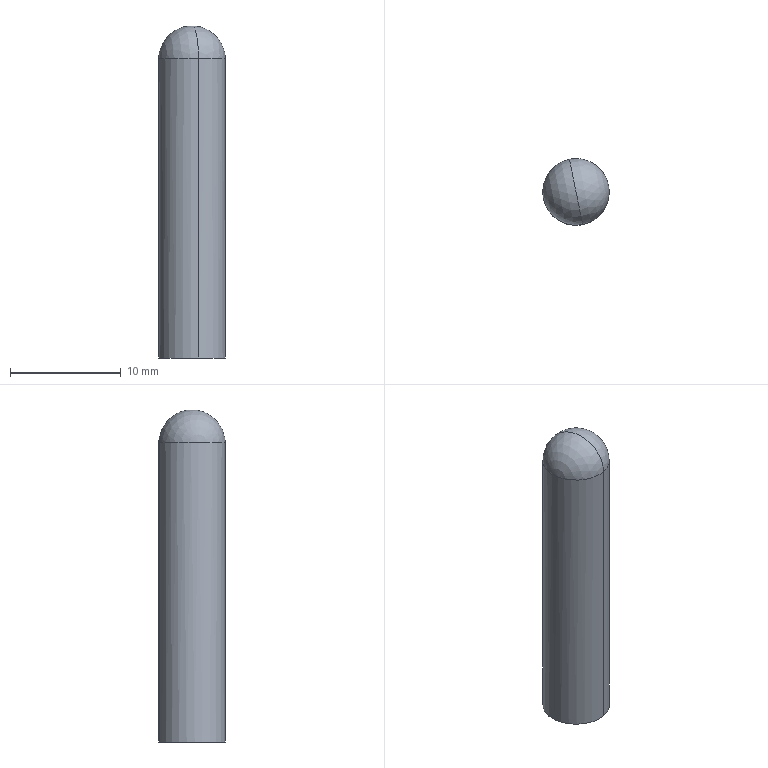Part | SolidWorks | features BaseBody 1 | 1 solid | 9 faces | box 6 x 6 x 30 mm | volume 732.824 mm3 | cylinder 4 | sphere 2 | cone 2 | plane 1 | commonest cylinder face diameters 2.5 x2 6 x2
STEP:
#1=CARTESIAN_POINT('',(-732.541,722.355,502.732));
#2=VERTEX_POINT('',#1);
#3=CARTESIAN_POINT('',(-732.541,722.355,529.732));
#4=VERTEX_POINT('',#3);
#5=CARTESIAN_POINT('',(-732.541,722.355,502.732));
#6=DIRECTION('',(0.,0.,1.));
#7=VECTOR('',#6,1000.);
#8=LINE('',#5,#7);
#9=EDGE_CURVE('',#2,#4,#8,.T.);
#10=ORIENTED_EDGE('',*,*,#9,.F.);
#11=CARTESIAN_POINT('',(-733.72,728.238,502.732));
#12=VERTEX_POINT('',#11);
#13=CARTESIAN_POINT('',(-733.131,725.297,502.732));
#14=DIRECTION('',(0.,0.,1.));
#15=DIRECTION('',(0.1964,-0.9805,0.));
#16=AXIS2_PLACEMENT_3D('',#13,#14,#15);
#17=CIRCLE('',#16,3.);
#18=EDGE_CURVE('',#2,#12,#17,.T.);
#19=ORIENTED_EDGE('',*,*,#18,.T.);
#20=CARTESIAN_POINT('',(-733.72,728.238,529.732));
#21=VERTEX_POINT('',#20);
#22=CARTESIAN_POINT('',(-733.72,728.238,529.732));
#23=DIRECTION('',(0.,0.,-1.));
#24=VECTOR('',#23,1000.);
#25=LINE('',#22,#24);
#26=EDGE_CURVE('',#21,#12,#25,.T.);
#27=ORIENTED_EDGE('',*,*,#26,.F.);
#28=CARTESIAN_POINT('',(-733.131,725.297,529.732));
#29=DIRECTION('',(0.,0.,-1.));
#30=DIRECTION('',(-0.1964,0.9805,0.));
#31=AXIS2_PLACEMENT_3D('',#28,#29,#30);
#32=CIRCLE('',#31,3.);
#33=EDGE_CURVE('',#21,#4,#32,.T.);
#34=ORIENTED_EDGE('',*,*,#33,.T.);
#35=EDGE_LOOP('',(#10,#19,#27,#34));
#36=FACE_OUTER_BOUND('',#35,.T.);
#37=CARTESIAN_POINT('',(-733.131,725.297,532.732));
#38=DIRECTION('',(0.,0.,-1.));
#39=DIRECTION('',(0.1964,-0.9805,0.));
#40=AXIS2_PLACEMENT_3D('',#37,#38,#39);
#41=CYLINDRICAL_SURFACE('',#40,3.);
#42=ADVANCED_FACE('',(#36),#41,.T.);
#43=CARTESIAN_POINT('',(-733.131,725.297,529.732));
#44=DIRECTION('',(0.9805,0.1964,0.));
#45=DIRECTION('',(-0.1964,0.9805,0.));
#46=AXIS2_PLACEMENT_3D('',#43,#44,#45);
#47=CIRCLE('',#46,3.);
#48=EDGE_CURVE('',#21,#4,#47,.T.);
#49=ORIENTED_EDGE('',*,*,#48,.T.);
#50=ORIENTED_EDGE('',*,*,#33,.F.);
#51=EDGE_LOOP('',(#49,#50));
#52=FACE_OUTER_BOUND('',#51,.T.);
#53=CARTESIAN_POINT('',(-733.131,725.297,529.732));
#54=DIRECTION('',(-0.9805,-0.1964,0.));
#55=DIRECTION('',(-0.1964,0.9805,0.));
#56=AXIS2_PLACEMENT_3D('',#53,#54,#55);
#57=SPHERICAL_SURFACE('',#56,3.);
#58=ADVANCED_FACE('',(#52),#57,.T.);
#59=CARTESIAN_POINT('',(-733.131,725.297,529.732));
#60=DIRECTION('',(0.,0.,-1.));
#61=DIRECTION('',(0.1964,-0.9805,0.));
#62=AXIS2_PLACEMENT_3D('',#59,#60,#61);
#63=CIRCLE('',#62,3.);
#64=EDGE_CURVE('',#4,#21,#63,.T.);
#65=ORIENTED_EDGE('',*,*,#64,.F.);
#66=ORIENTED_EDGE('',*,*,#48,.F.);
#67=EDGE_LOOP('',(#65,#66));
#68=FACE_OUTER_BOUND('',#67,.T.);
#69=CARTESIAN_POINT('',(-733.131,725.297,529.732));
#70=DIRECTION('',(-0.9805,-0.1964,0.));
#71=DIRECTION('',(-0.1964,0.9805,0.));
#72=AXIS2_PLACEMENT_3D('',#69,#70,#71);
#73=SPHERICAL_SURFACE('',#72,3.);
#74=ADVANCED_FACE('',(#68),#73,.T.);
#75=ORIENTED_EDGE('',*,*,#26,.T.);
#76=CARTESIAN_POINT('',(-733.131,725.297,502.732));
#77=DIRECTION('',(0.,0.,1.));
#78=DIRECTION('',(-0.1964,0.9805,0.));
#79=AXIS2_PLACEMENT_3D('',#76,#77,#78);
#80=CIRCLE('',#79,3.);
#81=EDGE_CURVE('',#12,#2,#80,.T.);
#82=ORIENTED_EDGE('',*,*,#81,.T.);
#83=ORIENTED_EDGE('',*,*,#9,.T.);
#84=ORIENTED_EDGE('',*,*,#64,.T.);
#85=EDGE_LOOP('',(#75,#82,#83,#84));
#86=FACE_OUTER_BOUND('',#85,.T.);
#87=CARTESIAN_POINT('',(-733.131,725.297,532.732));
#88=DIRECTION('',(0.,0.,-1.));
#89=DIRECTION('',(0.1964,-0.9805,0.));
#90=AXIS2_PLACEMENT_3D('',#87,#88,#89);
#91=CYLINDRICAL_SURFACE('',#90,3.);
#92=ADVANCED_FACE('',(#86),#91,.T.);
#93=ORIENTED_EDGE('',*,*,#18,.F.);
#94=ORIENTED_EDGE('',*,*,#81,.F.);
#95=EDGE_LOOP('',(#93,#94));
#96=FACE_OUTER_BOUND('',#95,.T.);
#97=CARTESIAN_POINT('',(-732.885,724.071,502.732));
#98=VERTEX_POINT('',#97);
#99=CARTESIAN_POINT('',(-733.376,726.523,502.732));
#100=VERTEX_POINT('',#99);
#101=CARTESIAN_POINT('',(-733.131,725.297,502.732));
#102=DIRECTION('',(0.,0.,-1.));
#103=DIRECTION('',(0.1964,-0.9805,0.));
#104=AXIS2_PLACEMENT_3D('',#101,#102,#103);
#105=CIRCLE('',#104,1.25);
#106=EDGE_CURVE('',#98,#100,#105,.T.);
#107=ORIENTED_EDGE('',*,*,#106,.F.);
#108=CARTESIAN_POINT('',(-733.131,725.297,502.732));
#109=DIRECTION('',(0.,0.,-1.));
#110=DIRECTION('',(-0.1964,0.9805,0.));
#111=AXIS2_PLACEMENT_3D('',#108,#109,#110);
#112=CIRCLE('',#111,1.25);
#113=EDGE_CURVE('',#100,#98,#112,.T.);
#114=ORIENTED_EDGE('',*,*,#113,.F.);
#115=EDGE_LOOP('',(#107,#114));
#116=FACE_BOUND('',#115,.T.);
#117=CARTESIAN_POINT('',(-733.131,725.297,502.732));
#118=DIRECTION('',(0.,0.,-1.));
#119=DIRECTION('',(0.1964,-0.9805,0.));
#120=AXIS2_PLACEMENT_3D('',#117,#118,#119);
#121=PLANE('',#120);
#122=ADVANCED_FACE('',(#96,#116),#121,.T.);
#123=CARTESIAN_POINT('',(-733.376,726.523,520.232));
#124=VERTEX_POINT('',#123);
#125=CARTESIAN_POINT('',(-733.376,726.523,520.232));
#126=DIRECTION('',(0.,0.,-1.));
#127=VECTOR('',#126,1000.);
#128=LINE('',#125,#127);
#129=EDGE_CURVE('',#124,#100,#128,.T.);
#130=ORIENTED_EDGE('',*,*,#129,.T.);
#131=ORIENTED_EDGE('',*,*,#113,.T.);
#132=CARTESIAN_POINT('',(-732.885,724.071,520.232));
#133=VERTEX_POINT('',#132);
#134=CARTESIAN_POINT('',(-732.885,724.071,502.732));
#135=DIRECTION('',(0.,0.,1.));
#136=VECTOR('',#135,1000.);
#137=LINE('',#134,#136);
#138=EDGE_CURVE('',#98,#133,#137,.T.);
#139=ORIENTED_EDGE('',*,*,#138,.T.);
#140=CARTESIAN_POINT('',(-733.131,725.297,520.232));
#141=DIRECTION('',(0.,0.,1.));
#142=DIRECTION('',(0.1964,-0.9805,0.));
#143=AXIS2_PLACEMENT_3D('',#140,#141,#142);
#144=CIRCLE('',#143,1.25);
#145=EDGE_CURVE('',#133,#124,#144,.T.);
#146=ORIENTED_EDGE('',*,*,#145,.T.);
#147=EDGE_LOOP('',(#130,#131,#139,#146));
#148=FACE_OUTER_BOUND('',#147,.T.);
#149=CARTESIAN_POINT('',(-733.131,725.297,512.732));
#150=DIRECTION('',(0.,0.,-1.));
#151=DIRECTION('',(0.1964,-0.9805,0.));
#152=AXIS2_PLACEMENT_3D('',#149,#150,#151);
#153=CYLINDRICAL_SURFACE('',#152,1.25);
#154=ADVANCED_FACE('',(#148),#153,.F.);
#155=ORIENTED_EDGE('',*,*,#145,.F.);
#156=CARTESIAN_POINT('',(-733.131,725.297,520.983));
#157=VERTEX_POINT('',#156);
#158=CARTESIAN_POINT('',(-733.131,725.297,520.983));
#159=DIRECTION('',(0.1683,-0.8405,-0.515));
#160=VECTOR('',#159,1000.);
#161=LINE('',#158,#160);
#162=EDGE_CURVE('',#157,#133,#161,.T.);
#163=ORIENTED_EDGE('',*,*,#162,.F.);
#164=CARTESIAN_POINT('',(-733.376,726.523,520.232));
#165=DIRECTION('',(0.1683,-0.8405,0.515));
#166=VECTOR('',#165,1000.);
#167=LINE('',#164,#166);
#168=EDGE_CURVE('',#124,#157,#167,.T.);
#169=ORIENTED_EDGE('',*,*,#168,.F.);
#170=EDGE_LOOP('',(#155,#163,#169));
#171=FACE_OUTER_BOUND('',#170,.T.);
#172=CARTESIAN_POINT('',(-733.131,725.297,520.598));
#173=DIRECTION('',(0.,0.,-1.));
#174=DIRECTION('',(-0.1964,0.9805,0.));
#175=AXIS2_PLACEMENT_3D('',#172,#173,#174);
#176=CONICAL_SURFACE('',#175,0.641,1.03);
#177=ADVANCED_FACE('',(#171),#176,.F.);
#178=CARTESIAN_POINT('',(-733.131,725.297,520.232));
#179=DIRECTION('',(0.,0.,1.));
#180=DIRECTION('',(-0.1964,0.9805,0.));
#181=AXIS2_PLACEMENT_3D('',#178,#179,#180);
#182=CIRCLE('',#181,1.25);
#183=EDGE_CURVE('',#124,#133,#182,.T.);
#184=ORIENTED_EDGE('',*,*,#183,.F.);
#185=ORIENTED_EDGE('',*,*,#168,.T.);
#186=ORIENTED_EDGE('',*,*,#162,.T.);
#187=EDGE_LOOP('',(#184,#185,#186));
#188=FACE_OUTER_BOUND('',#187,.T.);
#189=CARTESIAN_POINT('',(-733.131,725.297,520.598));
#190=DIRECTION('',(0.,0.,-1.));
#191=DIRECTION('',(-0.1964,0.9805,0.));
#192=AXIS2_PLACEMENT_3D('',#189,#190,#191);
#193=CONICAL_SURFACE('',#192,0.641,1.03);
#194=ADVANCED_FACE('',(#188),#193,.F.);
#195=ORIENTED_EDGE('',*,*,#138,.F.);
#196=ORIENTED_EDGE('',*,*,#106,.T.);
#197=ORIENTED_EDGE('',*,*,#129,.F.);
#198=ORIENTED_EDGE('',*,*,#183,.T.);
#199=EDGE_LOOP('',(#195,#196,#197,#198));
#200=FACE_OUTER_BOUND('',#199,.T.);
#201=CARTESIAN_POINT('',(-733.131,725.297,512.732));
#202=DIRECTION('',(0.,0.,-1.));
#203=DIRECTION('',(0.1964,-0.9805,0.));
#204=AXIS2_PLACEMENT_3D('',#201,#202,#203);
#205=CYLINDRICAL_SURFACE('',#204,1.25);
#206=ADVANCED_FACE('',(#200),#205,.F.);
#207=CLOSED_SHELL('',(#42,#58,#74,#92,#122,#154,#177,#194,#206));
#208=MANIFOLD_SOLID_BREP('',#207);
#209=CARTESIAN_POINT('',(0.,0.,0.));
#210=DIRECTION('',(0.,0.,1.));
#211=DIRECTION('',(1.,0.,0.));
#212=AXIS2_PLACEMENT_3D('',#209,#210,#211);
#213=(LENGTH_UNIT()NAMED_UNIT(*)SI_UNIT(.MILLI.,.METRE.));
#214=UNCERTAINTY_MEASURE_WITH_UNIT(LENGTH_MEASURE(0.00001),#213,'','');
#215=(NAMED_UNIT(*)PLANE_ANGLE_UNIT()SI_UNIT($,.RADIAN.));
#216=(NAMED_UNIT(*)SI_UNIT($,.STERADIAN.)SOLID_ANGLE_UNIT());
#217=(GEOMETRIC_REPRESENTATION_CONTEXT(3)GLOBAL_UNCERTAINTY_ASSIGNED_CONTEXT((#214))GLOBAL_UNIT_ASSIGNED_CONTEXT((#213,#215,#216))REPRESENTATION_CONTEXT('',''));
#218=ADVANCED_BREP_SHAPE_REPRESENTATION('',(#208,#212),#217);